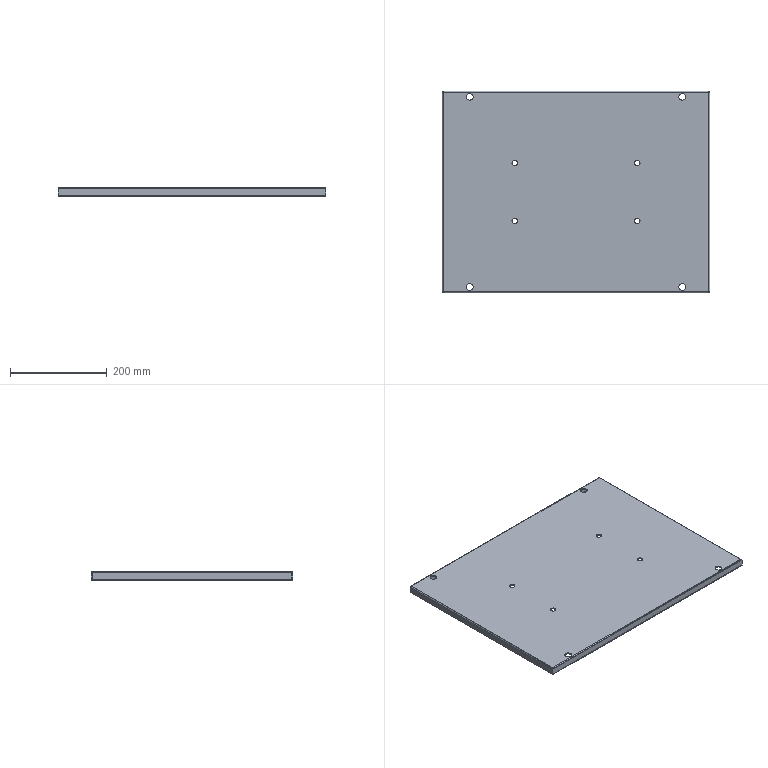Part | STEP file | TS-007-01 | 1 solid | 104 faces | box 554 x 418.001 x 17 mm | volume 565980 mm3 | plane 54 | cylinder 38 | spline 12 | commonest cylinder face diameters 0.4 x8 4.4 x8 11 x8 14 x8 18 x6